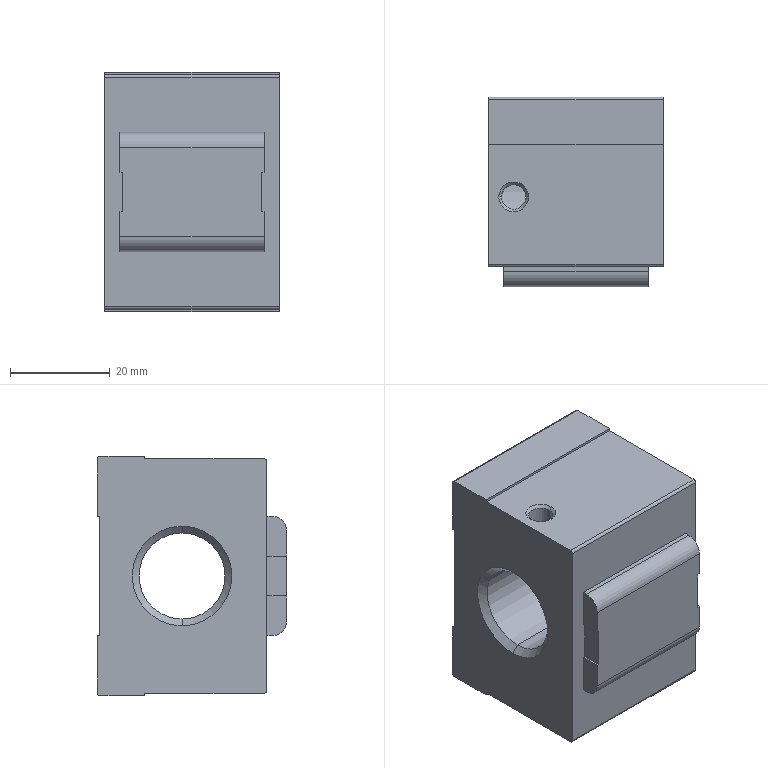Part | NX | features BREP 1 | 1 solid | 67 faces | box 35 x 38 x 48 mm | volume 49021 mm3 | plane 27 | cone 22 | cylinder 18 | commonest cylinder face diameters 4.917 x10 1 x4 6 x2 17.294 x2